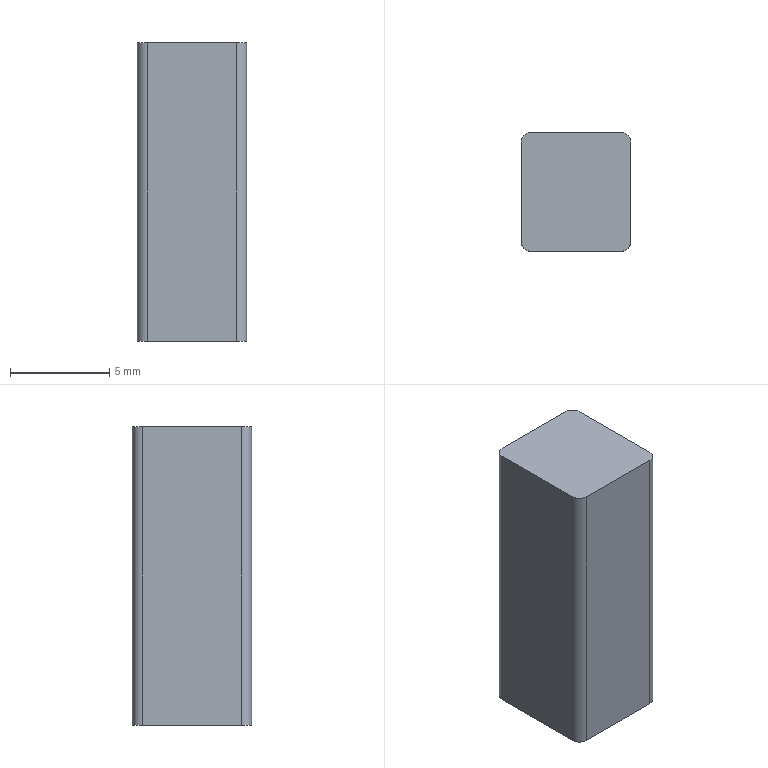Part | NX | features BREP 1 | 1 solid | 10 faces | box 5.5 x 6 x 15 mm | volume 491.781 mm3 | plane 6 | cylinder 4 | commonest cylinder face diameters 1 x4
STEP:
#1=CARTESIAN_POINT('',(-2.25,3.,-25.6));
#2=VERTEX_POINT('',#1);
#3=CARTESIAN_POINT('',(-2.75,2.5,-25.6));
#4=VERTEX_POINT('',#3);
#5=CARTESIAN_POINT('',(-2.25,2.5,-25.6));
#6=DIRECTION('',(0.,0.,1.));
#7=DIRECTION('',(1.,0.,0.));
#8=AXIS2_PLACEMENT_3D('',#5,#6,#7);
#9=CIRCLE('',#8,0.5);
#10=EDGE_CURVE('',#2,#4,#9,.T.);
#11=ORIENTED_EDGE('',*,*,#10,.F.);
#12=CARTESIAN_POINT('',(-2.25,3.,-40.6));
#13=VERTEX_POINT('',#12);
#14=CARTESIAN_POINT('',(-2.25,3.,-40.6));
#15=DIRECTION('',(0.,0.,1.));
#16=VECTOR('',#15,1000.);
#17=LINE('',#14,#16);
#18=EDGE_CURVE('',#13,#2,#17,.T.);
#19=ORIENTED_EDGE('',*,*,#18,.F.);
#20=CARTESIAN_POINT('',(-2.75,2.5,-40.6));
#21=VERTEX_POINT('',#20);
#22=CARTESIAN_POINT('',(-2.25,2.5,-40.6));
#23=DIRECTION('',(0.,0.,1.));
#24=DIRECTION('',(1.,0.,0.));
#25=AXIS2_PLACEMENT_3D('',#22,#23,#24);
#26=CIRCLE('',#25,0.5);
#27=EDGE_CURVE('',#13,#21,#26,.T.);
#28=ORIENTED_EDGE('',*,*,#27,.T.);
#29=CARTESIAN_POINT('',(-2.75,2.5,-40.6));
#30=DIRECTION('',(0.,0.,1.));
#31=VECTOR('',#30,1000.);
#32=LINE('',#29,#31);
#33=EDGE_CURVE('',#21,#4,#32,.T.);
#34=ORIENTED_EDGE('',*,*,#33,.T.);
#35=EDGE_LOOP('',(#11,#19,#28,#34));
#36=FACE_BOUND('',#35,.T.);
#37=CARTESIAN_POINT('',(-2.25,2.5,-40.6));
#38=DIRECTION('',(0.,0.,1.));
#39=DIRECTION('',(-1.,0.,0.));
#40=AXIS2_PLACEMENT_3D('',#37,#38,#39);
#41=CYLINDRICAL_SURFACE('',#40,0.5);
#42=ADVANCED_FACE('',(#36),#41,.T.);
#43=CARTESIAN_POINT('',(-2.75,-2.5,-25.6));
#44=VERTEX_POINT('',#43);
#45=CARTESIAN_POINT('',(-2.75,-2.5,-25.6));
#46=DIRECTION('',(0.,1.,0.));
#47=VECTOR('',#46,1000.);
#48=LINE('',#45,#47);
#49=EDGE_CURVE('',#44,#4,#48,.T.);
#50=ORIENTED_EDGE('',*,*,#49,.T.);
#51=ORIENTED_EDGE('',*,*,#33,.F.);
#52=CARTESIAN_POINT('',(-2.75,-2.5,-40.6));
#53=VERTEX_POINT('',#52);
#54=CARTESIAN_POINT('',(-2.75,-2.5,-40.6));
#55=DIRECTION('',(0.,1.,0.));
#56=VECTOR('',#55,1000.);
#57=LINE('',#54,#56);
#58=EDGE_CURVE('',#53,#21,#57,.T.);
#59=ORIENTED_EDGE('',*,*,#58,.F.);
#60=CARTESIAN_POINT('',(-2.75,-2.5,-40.6));
#61=DIRECTION('',(0.,0.,1.));
#62=VECTOR('',#61,1000.);
#63=LINE('',#60,#62);
#64=EDGE_CURVE('',#53,#44,#63,.T.);
#65=ORIENTED_EDGE('',*,*,#64,.T.);
#66=EDGE_LOOP('',(#50,#51,#59,#65));
#67=FACE_BOUND('',#66,.T.);
#68=CARTESIAN_POINT('',(-2.75,-2.5,-40.6));
#69=DIRECTION('',(1.,0.,0.));
#70=DIRECTION('',(0.,0.,1.));
#71=AXIS2_PLACEMENT_3D('',#68,#69,#70);
#72=PLANE('',#71);
#73=ADVANCED_FACE('',(#67),#72,.F.);
#74=CARTESIAN_POINT('',(-2.25,-3.,-25.6));
#75=VERTEX_POINT('',#74);
#76=CARTESIAN_POINT('',(-2.25,-2.5,-25.6));
#77=DIRECTION('',(0.,0.,1.));
#78=DIRECTION('',(1.,0.,0.));
#79=AXIS2_PLACEMENT_3D('',#76,#77,#78);
#80=CIRCLE('',#79,0.5);
#81=EDGE_CURVE('',#44,#75,#80,.T.);
#82=ORIENTED_EDGE('',*,*,#81,.F.);
#83=ORIENTED_EDGE('',*,*,#64,.F.);
#84=CARTESIAN_POINT('',(-2.25,-3.,-40.6));
#85=VERTEX_POINT('',#84);
#86=CARTESIAN_POINT('',(-2.25,-2.5,-40.6));
#87=DIRECTION('',(0.,0.,1.));
#88=DIRECTION('',(1.,0.,0.));
#89=AXIS2_PLACEMENT_3D('',#86,#87,#88);
#90=CIRCLE('',#89,0.5);
#91=EDGE_CURVE('',#53,#85,#90,.T.);
#92=ORIENTED_EDGE('',*,*,#91,.T.);
#93=CARTESIAN_POINT('',(-2.25,-3.,-40.6));
#94=DIRECTION('',(0.,0.,1.));
#95=VECTOR('',#94,1000.);
#96=LINE('',#93,#95);
#97=EDGE_CURVE('',#85,#75,#96,.T.);
#98=ORIENTED_EDGE('',*,*,#97,.T.);
#99=EDGE_LOOP('',(#82,#83,#92,#98));
#100=FACE_BOUND('',#99,.T.);
#101=CARTESIAN_POINT('',(-2.25,-2.5,-40.6));
#102=DIRECTION('',(0.,0.,1.));
#103=DIRECTION('',(-1.,0.,0.));
#104=AXIS2_PLACEMENT_3D('',#101,#102,#103);
#105=CYLINDRICAL_SURFACE('',#104,0.5);
#106=ADVANCED_FACE('',(#100),#105,.T.);
#107=CARTESIAN_POINT('',(2.25,-3.,-25.6));
#108=VERTEX_POINT('',#107);
#109=CARTESIAN_POINT('',(2.25,-3.,-25.6));
#110=DIRECTION('',(-1.,0.,0.));
#111=VECTOR('',#110,1000.);
#112=LINE('',#109,#111);
#113=EDGE_CURVE('',#108,#75,#112,.T.);
#114=ORIENTED_EDGE('',*,*,#113,.T.);
#115=ORIENTED_EDGE('',*,*,#97,.F.);
#116=CARTESIAN_POINT('',(2.25,-3.,-40.6));
#117=VERTEX_POINT('',#116);
#118=CARTESIAN_POINT('',(2.25,-3.,-40.6));
#119=DIRECTION('',(-1.,0.,0.));
#120=VECTOR('',#119,1000.);
#121=LINE('',#118,#120);
#122=EDGE_CURVE('',#117,#85,#121,.T.);
#123=ORIENTED_EDGE('',*,*,#122,.F.);
#124=CARTESIAN_POINT('',(2.25,-3.,-40.6));
#125=DIRECTION('',(0.,0.,1.));
#126=VECTOR('',#125,1000.);
#127=LINE('',#124,#126);
#128=EDGE_CURVE('',#117,#108,#127,.T.);
#129=ORIENTED_EDGE('',*,*,#128,.T.);
#130=EDGE_LOOP('',(#114,#115,#123,#129));
#131=FACE_BOUND('',#130,.T.);
#132=CARTESIAN_POINT('',(2.25,-3.,-40.6));
#133=DIRECTION('',(0.,1.,0.));
#134=DIRECTION('',(0.,0.,-1.));
#135=AXIS2_PLACEMENT_3D('',#132,#133,#134);
#136=PLANE('',#135);
#137=ADVANCED_FACE('',(#131),#136,.F.);
#138=CARTESIAN_POINT('',(2.75,-2.5,-25.6));
#139=VERTEX_POINT('',#138);
#140=CARTESIAN_POINT('',(2.25,-2.5,-25.6));
#141=DIRECTION('',(0.,0.,1.));
#142=DIRECTION('',(1.,0.,0.));
#143=AXIS2_PLACEMENT_3D('',#140,#141,#142);
#144=CIRCLE('',#143,0.5);
#145=EDGE_CURVE('',#108,#139,#144,.T.);
#146=ORIENTED_EDGE('',*,*,#145,.F.);
#147=ORIENTED_EDGE('',*,*,#128,.F.);
#148=CARTESIAN_POINT('',(2.75,-2.5,-40.6));
#149=VERTEX_POINT('',#148);
#150=CARTESIAN_POINT('',(2.25,-2.5,-40.6));
#151=DIRECTION('',(0.,0.,1.));
#152=DIRECTION('',(1.,0.,0.));
#153=AXIS2_PLACEMENT_3D('',#150,#151,#152);
#154=CIRCLE('',#153,0.5);
#155=EDGE_CURVE('',#117,#149,#154,.T.);
#156=ORIENTED_EDGE('',*,*,#155,.T.);
#157=CARTESIAN_POINT('',(2.75,-2.5,-40.6));
#158=DIRECTION('',(0.,0.,1.));
#159=VECTOR('',#158,1000.);
#160=LINE('',#157,#159);
#161=EDGE_CURVE('',#149,#139,#160,.T.);
#162=ORIENTED_EDGE('',*,*,#161,.T.);
#163=EDGE_LOOP('',(#146,#147,#156,#162));
#164=FACE_BOUND('',#163,.T.);
#165=CARTESIAN_POINT('',(2.25,-2.5,-40.6));
#166=DIRECTION('',(0.,0.,1.));
#167=DIRECTION('',(-1.,0.,0.));
#168=AXIS2_PLACEMENT_3D('',#165,#166,#167);
#169=CYLINDRICAL_SURFACE('',#168,0.5);
#170=ADVANCED_FACE('',(#164),#169,.T.);
#171=CARTESIAN_POINT('',(2.75,2.5,-25.6));
#172=VERTEX_POINT('',#171);
#173=CARTESIAN_POINT('',(2.75,2.5,-25.6));
#174=DIRECTION('',(0.,-1.,0.));
#175=VECTOR('',#174,1000.);
#176=LINE('',#173,#175);
#177=EDGE_CURVE('',#172,#139,#176,.T.);
#178=ORIENTED_EDGE('',*,*,#177,.T.);
#179=ORIENTED_EDGE('',*,*,#161,.F.);
#180=CARTESIAN_POINT('',(2.75,2.5,-40.6));
#181=VERTEX_POINT('',#180);
#182=CARTESIAN_POINT('',(2.75,2.5,-40.6));
#183=DIRECTION('',(0.,-1.,0.));
#184=VECTOR('',#183,1000.);
#185=LINE('',#182,#184);
#186=EDGE_CURVE('',#181,#149,#185,.T.);
#187=ORIENTED_EDGE('',*,*,#186,.F.);
#188=CARTESIAN_POINT('',(2.75,2.5,-40.6));
#189=DIRECTION('',(0.,0.,1.));
#190=VECTOR('',#189,1000.);
#191=LINE('',#188,#190);
#192=EDGE_CURVE('',#181,#172,#191,.T.);
#193=ORIENTED_EDGE('',*,*,#192,.T.);
#194=EDGE_LOOP('',(#178,#179,#187,#193));
#195=FACE_BOUND('',#194,.T.);
#196=CARTESIAN_POINT('',(2.75,2.5,-40.6));
#197=DIRECTION('',(-1.,0.,0.));
#198=DIRECTION('',(0.,0.,-1.));
#199=AXIS2_PLACEMENT_3D('',#196,#197,#198);
#200=PLANE('',#199);
#201=ADVANCED_FACE('',(#195),#200,.F.);
#202=CARTESIAN_POINT('',(2.25,3.,-25.6));
#203=VERTEX_POINT('',#202);
#204=CARTESIAN_POINT('',(2.25,2.5,-25.6));
#205=DIRECTION('',(0.,0.,1.));
#206=DIRECTION('',(1.,0.,0.));
#207=AXIS2_PLACEMENT_3D('',#204,#205,#206);
#208=CIRCLE('',#207,0.5);
#209=EDGE_CURVE('',#172,#203,#208,.T.);
#210=ORIENTED_EDGE('',*,*,#209,.F.);
#211=ORIENTED_EDGE('',*,*,#192,.F.);
#212=CARTESIAN_POINT('',(2.25,3.,-40.6));
#213=VERTEX_POINT('',#212);
#214=CARTESIAN_POINT('',(2.25,2.5,-40.6));
#215=DIRECTION('',(0.,0.,1.));
#216=DIRECTION('',(1.,0.,0.));
#217=AXIS2_PLACEMENT_3D('',#214,#215,#216);
#218=CIRCLE('',#217,0.5);
#219=EDGE_CURVE('',#181,#213,#218,.T.);
#220=ORIENTED_EDGE('',*,*,#219,.T.);
#221=CARTESIAN_POINT('',(2.25,3.,-40.6));
#222=DIRECTION('',(0.,0.,1.));
#223=VECTOR('',#222,1000.);
#224=LINE('',#221,#223);
#225=EDGE_CURVE('',#213,#203,#224,.T.);
#226=ORIENTED_EDGE('',*,*,#225,.T.);
#227=EDGE_LOOP('',(#210,#211,#220,#226));
#228=FACE_BOUND('',#227,.T.);
#229=CARTESIAN_POINT('',(2.25,2.5,-40.6));
#230=DIRECTION('',(0.,0.,1.));
#231=DIRECTION('',(-1.,0.,0.));
#232=AXIS2_PLACEMENT_3D('',#229,#230,#231);
#233=CYLINDRICAL_SURFACE('',#232,0.5);
#234=ADVANCED_FACE('',(#228),#233,.T.);
#235=CARTESIAN_POINT('',(-2.25,3.,-25.6));
#236=DIRECTION('',(1.,0.,0.));
#237=VECTOR('',#236,1000.);
#238=LINE('',#235,#237);
#239=EDGE_CURVE('',#2,#203,#238,.T.);
#240=ORIENTED_EDGE('',*,*,#239,.T.);
#241=ORIENTED_EDGE('',*,*,#225,.F.);
#242=CARTESIAN_POINT('',(-2.25,3.,-40.6));
#243=DIRECTION('',(1.,0.,0.));
#244=VECTOR('',#243,1000.);
#245=LINE('',#242,#244);
#246=EDGE_CURVE('',#13,#213,#245,.T.);
#247=ORIENTED_EDGE('',*,*,#246,.F.);
#248=ORIENTED_EDGE('',*,*,#18,.T.);
#249=EDGE_LOOP('',(#240,#241,#247,#248));
#250=FACE_BOUND('',#249,.T.);
#251=CARTESIAN_POINT('',(-2.25,3.,-40.6));
#252=DIRECTION('',(0.,-1.,0.));
#253=DIRECTION('',(0.,0.,1.));
#254=AXIS2_PLACEMENT_3D('',#251,#252,#253);
#255=PLANE('',#254);
#256=ADVANCED_FACE('',(#250),#255,.F.);
#257=ORIENTED_EDGE('',*,*,#27,.F.);
#258=ORIENTED_EDGE('',*,*,#246,.T.);
#259=ORIENTED_EDGE('',*,*,#219,.F.);
#260=ORIENTED_EDGE('',*,*,#186,.T.);
#261=ORIENTED_EDGE('',*,*,#155,.F.);
#262=ORIENTED_EDGE('',*,*,#122,.T.);
#263=ORIENTED_EDGE('',*,*,#91,.F.);
#264=ORIENTED_EDGE('',*,*,#58,.T.);
#265=EDGE_LOOP('',(#257,#258,#259,#260,#261,#262,#263,#264));
#266=FACE_BOUND('',#265,.T.);
#267=CARTESIAN_POINT('',(-2.25,2.5,-40.6));
#268=DIRECTION('',(0.,0.,1.));
#269=DIRECTION('',(-1.,0.,0.));
#270=AXIS2_PLACEMENT_3D('',#267,#268,#269);
#271=PLANE('',#270);
#272=ADVANCED_FACE('',(#266),#271,.F.);
#273=ORIENTED_EDGE('',*,*,#10,.T.);
#274=ORIENTED_EDGE('',*,*,#49,.F.);
#275=ORIENTED_EDGE('',*,*,#81,.T.);
#276=ORIENTED_EDGE('',*,*,#113,.F.);
#277=ORIENTED_EDGE('',*,*,#145,.T.);
#278=ORIENTED_EDGE('',*,*,#177,.F.);
#279=ORIENTED_EDGE('',*,*,#209,.T.);
#280=ORIENTED_EDGE('',*,*,#239,.F.);
#281=EDGE_LOOP('',(#273,#274,#275,#276,#277,#278,#279,#280));
#282=FACE_BOUND('',#281,.T.);
#283=CARTESIAN_POINT('',(-2.25,2.5,-25.6));
#284=DIRECTION('',(0.,0.,1.));
#285=DIRECTION('',(-1.,0.,0.));
#286=AXIS2_PLACEMENT_3D('',#283,#284,#285);
#287=PLANE('',#286);
#288=ADVANCED_FACE('',(#282),#287,.T.);
#289=CLOSED_SHELL('',(#42,#73,#106,#137,#170,#201,#234,#256,#272,#288));
#290=MANIFOLD_SOLID_BREP('',#289);
#291=(LENGTH_UNIT()NAMED_UNIT(*)SI_UNIT(.MILLI.,.METRE.));
#292=UNCERTAINTY_MEASURE_WITH_UNIT(LENGTH_MEASURE(0.00001),#291,'','');
#293=(NAMED_UNIT(*)PLANE_ANGLE_UNIT()SI_UNIT($,.RADIAN.));
#294=(NAMED_UNIT(*)SI_UNIT($,.STERADIAN.)SOLID_ANGLE_UNIT());
#295=(GEOMETRIC_REPRESENTATION_CONTEXT(3)GLOBAL_UNCERTAINTY_ASSIGNED_CONTEXT((#292))GLOBAL_UNIT_ASSIGNED_CONTEXT((#291,#293,#294))REPRESENTATION_CONTEXT('',''));
#296=ADVANCED_BREP_SHAPE_REPRESENTATION('',(#290),#295);